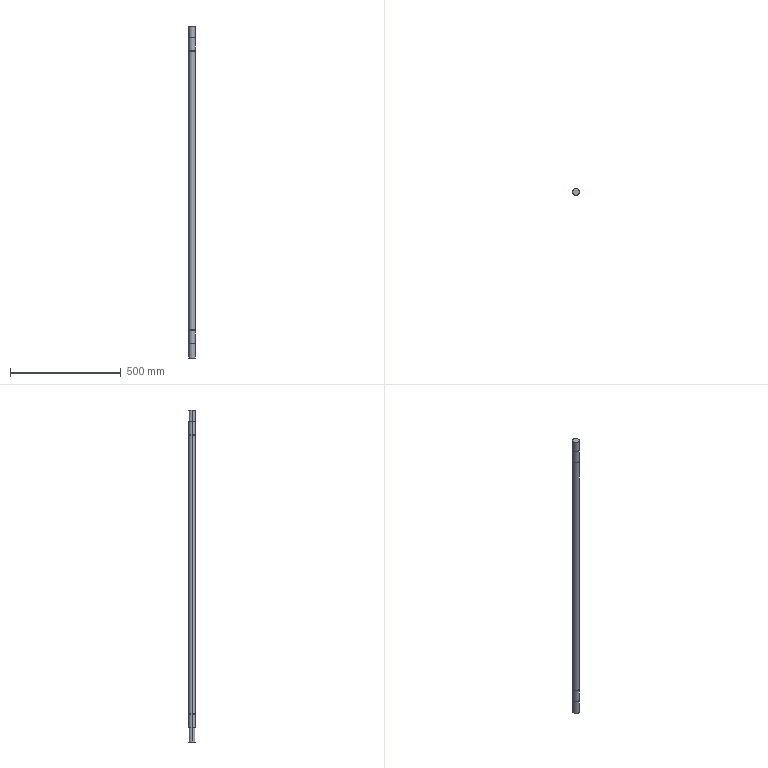Part | SolidWorks | features Extrusion 1, HoleWzd 1, ICE 1, LPattern 1, RevCut 1 | 1 solid | 44 faces | box 30 x 30 x 1500 mm | volume 1054135 mm3 | cylinder 26 | plane 16 | cone 2 | commonest cylinder face diameters 30 x10 28.6 x8 10 x6 6.8 x2
STEP:
#1=CARTESIAN_POINT('',(3.4,0.,19.75));
#2=VERTEX_POINT('',#1);
#3=CARTESIAN_POINT('',(-3.4,0.,19.75));
#4=VERTEX_POINT('',#3);
#5=CARTESIAN_POINT('',(0.,0.,19.75));
#6=DIRECTION('',(0.,0.,-1.));
#7=DIRECTION('',(-1.,0.,0.));
#8=AXIS2_PLACEMENT_3D('',#5,#6,#7);
#9=CIRCLE('',#8,3.4);
#10=EDGE_CURVE('',#2,#4,#9,.T.);
#11=ORIENTED_EDGE('',*,*,#10,.F.);
#12=CARTESIAN_POINT('',(3.4,0.,0.));
#13=VERTEX_POINT('',#12);
#14=CARTESIAN_POINT('',(3.4,0.,0.));
#15=DIRECTION('',(0.,0.,-1.));
#16=VECTOR('',#15,1000.);
#17=LINE('',#14,#16);
#18=EDGE_CURVE('',#2,#13,#17,.T.);
#19=ORIENTED_EDGE('',*,*,#18,.T.);
#20=CARTESIAN_POINT('',(-3.4,0.,0.));
#21=VERTEX_POINT('',#20);
#22=CARTESIAN_POINT('',(0.,0.,0.));
#23=DIRECTION('',(0.,0.,-1.));
#24=DIRECTION('',(-1.,0.,0.));
#25=AXIS2_PLACEMENT_3D('',#22,#23,#24);
#26=CIRCLE('',#25,3.4);
#27=EDGE_CURVE('',#13,#21,#26,.T.);
#28=ORIENTED_EDGE('',*,*,#27,.T.);
#29=CARTESIAN_POINT('',(-3.4,0.,0.));
#30=DIRECTION('',(0.,0.,-1.));
#31=VECTOR('',#30,1000.);
#32=LINE('',#29,#31);
#33=EDGE_CURVE('',#4,#21,#32,.T.);
#34=ORIENTED_EDGE('',*,*,#33,.F.);
#35=EDGE_LOOP('',(#11,#19,#28,#34));
#36=FACE_OUTER_BOUND('',#35,.T.);
#37=CARTESIAN_POINT('',(0.,0.,0.));
#38=DIRECTION('',(0.,0.,-1.));
#39=DIRECTION('',(-1.,0.,0.));
#40=AXIS2_PLACEMENT_3D('',#37,#38,#39);
#41=CYLINDRICAL_SURFACE('',#40,3.4);
#42=ADVANCED_FACE('',(#36),#41,.F.);
#43=CARTESIAN_POINT('',(0.,0.,21.793));
#44=VERTEX_POINT('',#43);
#45=CARTESIAN_POINT('',(-3.4,0.,19.75));
#46=DIRECTION('',(-0.8572,0.,-0.515));
#47=VECTOR('',#46,1000.);
#48=LINE('',#45,#47);
#49=EDGE_CURVE('',#44,#4,#48,.T.);
#50=ORIENTED_EDGE('',*,*,#49,.F.);
#51=CARTESIAN_POINT('',(3.4,0.,19.75));
#52=DIRECTION('',(0.8572,0.,-0.515));
#53=VECTOR('',#52,1000.);
#54=LINE('',#51,#53);
#55=EDGE_CURVE('',#44,#2,#54,.T.);
#56=ORIENTED_EDGE('',*,*,#55,.T.);
#57=ORIENTED_EDGE('',*,*,#10,.T.);
#58=EDGE_LOOP('',(#50,#56,#57));
#59=FACE_OUTER_BOUND('',#58,.T.);
#60=CARTESIAN_POINT('',(0.,0.,19.75));
#61=DIRECTION('',(0.,0.,-1.));
#62=DIRECTION('',(-1.,0.,0.));
#63=AXIS2_PLACEMENT_3D('',#60,#61,#62);
#64=CONICAL_SURFACE('',#63,3.4,1.03);
#65=ADVANCED_FACE('',(#59),#64,.F.);
#66=CARTESIAN_POINT('',(-15.,0.,63.9));
#67=VERTEX_POINT('',#66);
#68=CARTESIAN_POINT('',(15.,0.,63.9));
#69=VERTEX_POINT('',#68);
#70=CARTESIAN_POINT('',(0.,0.,63.9));
#71=DIRECTION('',(0.,0.,-1.));
#72=DIRECTION('',(0.,1.,0.));
#73=AXIS2_PLACEMENT_3D('',#70,#71,#72);
#74=CIRCLE('',#73,15.);
#75=EDGE_CURVE('',#67,#69,#74,.T.);
#76=ORIENTED_EDGE('',*,*,#75,.T.);
#77=CARTESIAN_POINT('',(15.,0.,0.));
#78=VERTEX_POINT('',#77);
#79=CARTESIAN_POINT('',(15.,0.,1500.));
#80=DIRECTION('',(0.,0.,-1.));
#81=VECTOR('',#80,1000.);
#82=LINE('',#79,#81);
#83=EDGE_CURVE('',#69,#78,#82,.T.);
#84=ORIENTED_EDGE('',*,*,#83,.T.);
#85=CARTESIAN_POINT('',(-15.,0.,0.));
#86=VERTEX_POINT('',#85);
#87=CARTESIAN_POINT('',(0.,0.,0.));
#88=DIRECTION('',(0.,0.,1.));
#89=DIRECTION('',(1.,0.,0.));
#90=AXIS2_PLACEMENT_3D('',#87,#88,#89);
#91=CIRCLE('',#90,15.);
#92=EDGE_CURVE('',#78,#86,#91,.T.);
#93=ORIENTED_EDGE('',*,*,#92,.T.);
#94=CARTESIAN_POINT('',(-15.,0.,1500.));
#95=DIRECTION('',(0.,0.,-1.));
#96=VECTOR('',#95,1000.);
#97=LINE('',#94,#96);
#98=EDGE_CURVE('',#67,#86,#97,.T.);
#99=ORIENTED_EDGE('',*,*,#98,.F.);
#100=EDGE_LOOP('',(#76,#84,#93,#99));
#101=FACE_OUTER_BOUND('',#100,.T.);
#102=CARTESIAN_POINT('',(0.,0.,1500.));
#103=DIRECTION('',(0.,0.,-1.));
#104=DIRECTION('',(-1.,0.,0.));
#105=AXIS2_PLACEMENT_3D('',#102,#103,#104);
#106=CYLINDRICAL_SURFACE('',#105,15.);
#107=ADVANCED_FACE('',(#101),#106,.T.);
#108=CARTESIAN_POINT('',(0.,14.3,65.5));
#109=VERTEX_POINT('',#108);
#110=CARTESIAN_POINT('',(0.,-14.3,65.5));
#111=VERTEX_POINT('',#110);
#112=CARTESIAN_POINT('',(0.,0.,65.5));
#113=DIRECTION('',(0.,0.,-1.));
#114=DIRECTION('',(0.,1.,0.));
#115=AXIS2_PLACEMENT_3D('',#112,#113,#114);
#116=CIRCLE('',#115,14.3);
#117=EDGE_CURVE('',#109,#111,#116,.T.);
#118=ORIENTED_EDGE('',*,*,#117,.T.);
#119=CARTESIAN_POINT('',(0.,-14.3,63.9));
#120=VERTEX_POINT('',#119);
#121=CARTESIAN_POINT('',(0.,-14.3,123.));
#122=DIRECTION('',(0.,0.,-1.));
#123=VECTOR('',#122,1000.);
#124=LINE('',#121,#123);
#125=EDGE_CURVE('',#111,#120,#124,.T.);
#126=ORIENTED_EDGE('',*,*,#125,.T.);
#127=CARTESIAN_POINT('',(0.,14.3,63.9));
#128=VERTEX_POINT('',#127);
#129=CARTESIAN_POINT('',(0.,0.,63.9));
#130=DIRECTION('',(0.,0.,-1.));
#131=DIRECTION('',(0.,1.,0.));
#132=AXIS2_PLACEMENT_3D('',#129,#130,#131);
#133=CIRCLE('',#132,14.3);
#134=EDGE_CURVE('',#128,#120,#133,.T.);
#135=ORIENTED_EDGE('',*,*,#134,.F.);
#136=CARTESIAN_POINT('',(0.,14.3,123.));
#137=DIRECTION('',(0.,0.,-1.));
#138=VECTOR('',#137,1000.);
#139=LINE('',#136,#138);
#140=EDGE_CURVE('',#109,#128,#139,.T.);
#141=ORIENTED_EDGE('',*,*,#140,.F.);
#142=EDGE_LOOP('',(#118,#126,#135,#141));
#143=FACE_OUTER_BOUND('',#142,.T.);
#144=CARTESIAN_POINT('',(0.,0.,123.));
#145=DIRECTION('',(0.,0.,-1.));
#146=DIRECTION('',(0.,1.,0.));
#147=AXIS2_PLACEMENT_3D('',#144,#145,#146);
#148=CYLINDRICAL_SURFACE('',#147,14.3);
#149=ADVANCED_FACE('',(#143),#148,.T.);
#150=CARTESIAN_POINT('',(-15.,0.,125.5));
#151=VERTEX_POINT('',#150);
#152=CARTESIAN_POINT('',(15.,0.,125.5));
#153=VERTEX_POINT('',#152);
#154=CARTESIAN_POINT('',(0.,0.,125.5));
#155=DIRECTION('',(0.,0.,-1.));
#156=DIRECTION('',(0.,1.,0.));
#157=AXIS2_PLACEMENT_3D('',#154,#155,#156);
#158=CIRCLE('',#157,15.);
#159=EDGE_CURVE('',#151,#153,#158,.T.);
#160=ORIENTED_EDGE('',*,*,#159,.T.);
#161=CARTESIAN_POINT('',(15.,0.,123.));
#162=VERTEX_POINT('',#161);
#163=CARTESIAN_POINT('',(15.,0.,1500.));
#164=DIRECTION('',(0.,0.,-1.));
#165=VECTOR('',#164,1000.);
#166=LINE('',#163,#165);
#167=EDGE_CURVE('',#153,#162,#166,.T.);
#168=ORIENTED_EDGE('',*,*,#167,.T.);
#169=CARTESIAN_POINT('',(14.142,5.,118.));
#170=VERTEX_POINT('',#169);
#171=CARTESIAN_POINT('',(14.142,5.,118.));
#172=CARTESIAN_POINT('',(14.142,5.,118.33));
#173=CARTESIAN_POINT('',(14.154,4.968,118.656));
#174=CARTESIAN_POINT('',(14.187,4.871,119.14));
#175=CARTESIAN_POINT('',(14.201,4.83,119.302));
#176=CARTESIAN_POINT('',(14.233,4.734,119.617));
#177=CARTESIAN_POINT('',(14.252,4.679,119.771));
#178=CARTESIAN_POINT('',(14.313,4.491,120.222));
#179=CARTESIAN_POINT('',(14.361,4.336,120.511));
#180=CARTESIAN_POINT('',(14.466,3.971,121.055));
#181=CARTESIAN_POINT('',(14.522,3.765,121.305));
#182=CARTESIAN_POINT('',(14.633,3.307,121.764));
#183=CARTESIAN_POINT('',(14.689,3.052,121.974));
#184=CARTESIAN_POINT('',(14.791,2.512,122.336));
#185=CARTESIAN_POINT('',(14.837,2.226,122.489));
#186=CARTESIAN_POINT('',(14.896,1.772,122.678));
#187=CARTESIAN_POINT('',(14.914,1.616,122.735));
#188=CARTESIAN_POINT('',(14.944,1.301,122.831));
#189=CARTESIAN_POINT('',(14.957,1.142,122.871));
#190=CARTESIAN_POINT('',(14.989,0.6599,122.967));
#191=CARTESIAN_POINT('',(15.,0.3329,123.));
#192=CARTESIAN_POINT('',(15.,0.,123.));
#193=B_SPLINE_CURVE_WITH_KNOTS('',3,(#171,#172,#173,#174,#175,#176,#177,#178,#179,#180,#181,#182,#183,#184,#185,#186,#187,#188,#189,#190,#191,#192),.UNSPECIFIED.,.F.,.F.,(4,2,2,2,2,2,2,2,2,2,4),(0.02362,0.0246,0.02509,0.02558,0.02657,0.02755,0.02854,0.02952,0.03001,0.0305,0.03149),.UNSPECIFIED.);
#194=EDGE_CURVE('',#170,#162,#193,.T.);
#195=ORIENTED_EDGE('',*,*,#194,.F.);
#196=CARTESIAN_POINT('',(14.142,5.,73.));
#197=VERTEX_POINT('',#196);
#198=CARTESIAN_POINT('',(14.142,5.,1500.));
#199=DIRECTION('',(0.,0.,1.));
#200=VECTOR('',#199,1000.);
#201=LINE('',#198,#200);
#202=EDGE_CURVE('',#197,#170,#201,.T.);
#203=ORIENTED_EDGE('',*,*,#202,.F.);
#204=CARTESIAN_POINT('',(15.,0.,68.));
#205=VERTEX_POINT('',#204);
#206=CARTESIAN_POINT('',(15.,0.,68.));
#207=CARTESIAN_POINT('',(15.,0.3279,68.));
#208=CARTESIAN_POINT('',(14.989,0.658,68.032));
#209=CARTESIAN_POINT('',(14.947,1.307,68.162));
#210=CARTESIAN_POINT('',(14.915,1.619,68.258));
#211=CARTESIAN_POINT('',(14.838,2.223,68.509));
#212=CARTESIAN_POINT('',(14.79,2.515,68.666));
#213=CARTESIAN_POINT('',(14.688,3.055,69.028));
#214=CARTESIAN_POINT('',(14.633,3.305,69.234));
#215=CARTESIAN_POINT('',(14.521,3.767,69.696));
#216=CARTESIAN_POINT('',(14.465,3.974,69.949));
#217=CARTESIAN_POINT('',(14.361,4.335,70.487));
#218=CARTESIAN_POINT('',(14.313,4.49,70.776));
#219=CARTESIAN_POINT('',(14.231,4.743,71.383));
#220=CARTESIAN_POINT('',(14.199,4.838,71.695));
#221=CARTESIAN_POINT('',(14.154,4.967,72.337));
#222=CARTESIAN_POINT('',(14.142,5.,72.671));
#223=CARTESIAN_POINT('',(14.142,5.,73.));
#224=B_SPLINE_CURVE_WITH_KNOTS('',3,(#206,#207,#208,#209,#210,#211,#212,#213,#214,#215,#216,#217,#218,#219,#220,#221,#222,#223),.UNSPECIFIED.,.F.,.F.,(4,2,2,2,2,2,2,2,4),(0.01575,0.01673,0.01771,0.0187,0.01968,0.02066,0.02165,0.02263,0.02362),.UNSPECIFIED.);
#225=EDGE_CURVE('',#205,#197,#224,.T.);
#226=ORIENTED_EDGE('',*,*,#225,.F.);
#227=CARTESIAN_POINT('',(15.,0.,65.5));
#228=VERTEX_POINT('',#227);
#229=CARTESIAN_POINT('',(15.,0.,1500.));
#230=DIRECTION('',(0.,0.,-1.));
#231=VECTOR('',#230,1000.);
#232=LINE('',#229,#231);
#233=EDGE_CURVE('',#205,#228,#232,.T.);
#234=ORIENTED_EDGE('',*,*,#233,.T.);
#235=CARTESIAN_POINT('',(-15.,0.,65.5));
#236=VERTEX_POINT('',#235);
#237=CARTESIAN_POINT('',(0.,0.,65.5));
#238=DIRECTION('',(0.,0.,-1.));
#239=DIRECTION('',(0.,1.,0.));
#240=AXIS2_PLACEMENT_3D('',#237,#238,#239);
#241=CIRCLE('',#240,15.);
#242=EDGE_CURVE('',#236,#228,#241,.T.);
#243=ORIENTED_EDGE('',*,*,#242,.F.);
#244=CARTESIAN_POINT('',(-15.,0.,1500.));
#245=DIRECTION('',(0.,0.,-1.));
#246=VECTOR('',#245,1000.);
#247=LINE('',#244,#246);
#248=EDGE_CURVE('',#151,#236,#247,.T.);
#249=ORIENTED_EDGE('',*,*,#248,.F.);
#250=EDGE_LOOP('',(#160,#168,#195,#203,#226,#234,#243,#249));
#251=FACE_OUTER_BOUND('',#250,.T.);
#252=CARTESIAN_POINT('',(0.,0.,1500.));
#253=DIRECTION('',(0.,0.,-1.));
#254=DIRECTION('',(-1.,0.,0.));
#255=AXIS2_PLACEMENT_3D('',#252,#253,#254);
#256=CYLINDRICAL_SURFACE('',#255,15.);
#257=ADVANCED_FACE('',(#251),#256,.T.);
#258=ORIENTED_EDGE('',*,*,#194,.T.);
#259=CARTESIAN_POINT('',(10.,0.,123.));
#260=VERTEX_POINT('',#259);
#261=CARTESIAN_POINT('',(15.,0.,123.));
#262=DIRECTION('',(-1.,0.,0.));
#263=VECTOR('',#262,1000.);
#264=LINE('',#261,#263);
#265=EDGE_CURVE('',#162,#260,#264,.T.);
#266=ORIENTED_EDGE('',*,*,#265,.T.);
#267=CARTESIAN_POINT('',(10.,5.,118.));
#268=VERTEX_POINT('',#267);
#269=CARTESIAN_POINT('',(10.,0.,118.));
#270=DIRECTION('',(1.,0.,0.));
#271=DIRECTION('',(0.,0.,-1.));
#272=AXIS2_PLACEMENT_3D('',#269,#270,#271);
#273=CIRCLE('',#272,5.);
#274=EDGE_CURVE('',#268,#260,#273,.T.);
#275=ORIENTED_EDGE('',*,*,#274,.F.);
#276=CARTESIAN_POINT('',(15.,5.,118.));
#277=DIRECTION('',(-1.,0.,0.));
#278=VECTOR('',#277,1000.);
#279=LINE('',#276,#278);
#280=EDGE_CURVE('',#170,#268,#279,.T.);
#281=ORIENTED_EDGE('',*,*,#280,.F.);
#282=EDGE_LOOP('',(#258,#266,#275,#281));
#283=FACE_OUTER_BOUND('',#282,.T.);
#284=CARTESIAN_POINT('',(15.,0.,118.));
#285=DIRECTION('',(-1.,0.,0.));
#286=DIRECTION('',(0.,0.,1.));
#287=AXIS2_PLACEMENT_3D('',#284,#285,#286);
#288=CYLINDRICAL_SURFACE('',#287,5.);
#289=ADVANCED_FACE('',(#283),#288,.F.);
#290=CARTESIAN_POINT('',(0.,14.3,127.1));
#291=VERTEX_POINT('',#290);
#292=CARTESIAN_POINT('',(0.,-14.3,127.1));
#293=VERTEX_POINT('',#292);
#294=CARTESIAN_POINT('',(0.,0.,127.1));
#295=DIRECTION('',(0.,0.,-1.));
#296=DIRECTION('',(0.,1.,0.));
#297=AXIS2_PLACEMENT_3D('',#294,#295,#296);
#298=CIRCLE('',#297,14.3);
#299=EDGE_CURVE('',#291,#293,#298,.T.);
#300=ORIENTED_EDGE('',*,*,#299,.T.);
#301=CARTESIAN_POINT('',(0.,-14.3,125.5));
#302=VERTEX_POINT('',#301);
#303=CARTESIAN_POINT('',(0.,-14.3,123.));
#304=DIRECTION('',(0.,0.,-1.));
#305=VECTOR('',#304,1000.);
#306=LINE('',#303,#305);
#307=EDGE_CURVE('',#293,#302,#306,.T.);
#308=ORIENTED_EDGE('',*,*,#307,.T.);
#309=CARTESIAN_POINT('',(0.,14.3,125.5));
#310=VERTEX_POINT('',#309);
#311=CARTESIAN_POINT('',(0.,0.,125.5));
#312=DIRECTION('',(0.,0.,-1.));
#313=DIRECTION('',(0.,1.,0.));
#314=AXIS2_PLACEMENT_3D('',#311,#312,#313);
#315=CIRCLE('',#314,14.3);
#316=EDGE_CURVE('',#310,#302,#315,.T.);
#317=ORIENTED_EDGE('',*,*,#316,.F.);
#318=CARTESIAN_POINT('',(0.,14.3,123.));
#319=DIRECTION('',(0.,0.,-1.));
#320=VECTOR('',#319,1000.);
#321=LINE('',#318,#320);
#322=EDGE_CURVE('',#291,#310,#321,.T.);
#323=ORIENTED_EDGE('',*,*,#322,.F.);
#324=EDGE_LOOP('',(#300,#308,#317,#323));
#325=FACE_OUTER_BOUND('',#324,.T.);
#326=CARTESIAN_POINT('',(0.,0.,123.));
#327=DIRECTION('',(0.,0.,-1.));
#328=DIRECTION('',(0.,1.,0.));
#329=AXIS2_PLACEMENT_3D('',#326,#327,#328);
#330=CYLINDRICAL_SURFACE('',#329,14.3);
#331=ADVANCED_FACE('',(#325),#330,.T.);
#332=CARTESIAN_POINT('',(15.,0.,1500.));
#333=VERTEX_POINT('',#332);
#334=CARTESIAN_POINT('',(-15.,0.,1500.));
#335=VERTEX_POINT('',#334);
#336=CARTESIAN_POINT('',(0.,0.,1500.));
#337=DIRECTION('',(0.,0.,1.));
#338=DIRECTION('',(1.,0.,0.));
#339=AXIS2_PLACEMENT_3D('',#336,#337,#338);
#340=CIRCLE('',#339,15.);
#341=EDGE_CURVE('',#333,#335,#340,.T.);
#342=ORIENTED_EDGE('',*,*,#341,.F.);
#343=CARTESIAN_POINT('',(15.,0.,1449.1));
#344=VERTEX_POINT('',#343);
#345=CARTESIAN_POINT('',(15.,0.,1500.));
#346=DIRECTION('',(0.,0.,-1.));
#347=VECTOR('',#346,1000.);
#348=LINE('',#345,#347);
#349=EDGE_CURVE('',#333,#344,#348,.T.);
#350=ORIENTED_EDGE('',*,*,#349,.T.);
#351=CARTESIAN_POINT('',(-15.,0.,1449.1));
#352=VERTEX_POINT('',#351);
#353=CARTESIAN_POINT('',(0.,0.,1449.1));
#354=DIRECTION('',(0.,0.,-1.));
#355=DIRECTION('',(0.,1.,0.));
#356=AXIS2_PLACEMENT_3D('',#353,#354,#355);
#357=CIRCLE('',#356,15.);
#358=EDGE_CURVE('',#352,#344,#357,.T.);
#359=ORIENTED_EDGE('',*,*,#358,.F.);
#360=CARTESIAN_POINT('',(-15.,0.,1500.));
#361=DIRECTION('',(0.,0.,-1.));
#362=VECTOR('',#361,1000.);
#363=LINE('',#360,#362);
#364=EDGE_CURVE('',#335,#352,#363,.T.);
#365=ORIENTED_EDGE('',*,*,#364,.F.);
#366=EDGE_LOOP('',(#342,#350,#359,#365));
#367=FACE_OUTER_BOUND('',#366,.T.);
#368=CARTESIAN_POINT('',(0.,0.,1500.));
#369=DIRECTION('',(0.,0.,-1.));
#370=DIRECTION('',(-1.,0.,0.));
#371=AXIS2_PLACEMENT_3D('',#368,#369,#370);
#372=CYLINDRICAL_SURFACE('',#371,15.);
#373=ADVANCED_FACE('',(#367),#372,.T.);
#374=CARTESIAN_POINT('',(0.,14.3,1449.1));
#375=VERTEX_POINT('',#374);
#376=CARTESIAN_POINT('',(0.,-14.3,1449.1));
#377=VERTEX_POINT('',#376);
#378=CARTESIAN_POINT('',(0.,0.,1449.1));
#379=DIRECTION('',(0.,0.,-1.));
#380=DIRECTION('',(0.,1.,0.));
#381=AXIS2_PLACEMENT_3D('',#378,#379,#380);
#382=CIRCLE('',#381,14.3);
#383=EDGE_CURVE('',#375,#377,#382,.T.);
#384=ORIENTED_EDGE('',*,*,#383,.T.);
#385=CARTESIAN_POINT('',(0.,-14.3,1447.5));
#386=VERTEX_POINT('',#385);
#387=CARTESIAN_POINT('',(0.,-14.3,1445.));
#388=DIRECTION('',(0.,0.,-1.));
#389=VECTOR('',#388,1000.);
#390=LINE('',#387,#389);
#391=EDGE_CURVE('',#377,#386,#390,.T.);
#392=ORIENTED_EDGE('',*,*,#391,.T.);
#393=CARTESIAN_POINT('',(0.,14.3,1447.5));
#394=VERTEX_POINT('',#393);
#395=CARTESIAN_POINT('',(0.,0.,1447.5));
#396=DIRECTION('',(0.,0.,-1.));
#397=DIRECTION('',(0.,1.,0.));
#398=AXIS2_PLACEMENT_3D('',#395,#396,#397);
#399=CIRCLE('',#398,14.3);
#400=EDGE_CURVE('',#394,#386,#399,.T.);
#401=ORIENTED_EDGE('',*,*,#400,.F.);
#402=CARTESIAN_POINT('',(0.,14.3,1445.));
#403=DIRECTION('',(0.,0.,-1.));
#404=VECTOR('',#403,1000.);
#405=LINE('',#402,#404);
#406=EDGE_CURVE('',#375,#394,#405,.T.);
#407=ORIENTED_EDGE('',*,*,#406,.F.);
#408=EDGE_LOOP('',(#384,#392,#401,#407));
#409=FACE_OUTER_BOUND('',#408,.T.);
#410=CARTESIAN_POINT('',(0.,0.,1445.));
#411=DIRECTION('',(0.,0.,-1.));
#412=DIRECTION('',(0.,1.,0.));
#413=AXIS2_PLACEMENT_3D('',#410,#411,#412);
#414=CYLINDRICAL_SURFACE('',#413,14.3);
#415=ADVANCED_FACE('',(#409),#414,.T.);
#416=CARTESIAN_POINT('',(0.,14.3,1387.5));
#417=VERTEX_POINT('',#416);
#418=CARTESIAN_POINT('',(0.,-14.3,1387.5));
#419=VERTEX_POINT('',#418);
#420=CARTESIAN_POINT('',(0.,0.,1387.5));
#421=DIRECTION('',(0.,0.,-1.));
#422=DIRECTION('',(0.,1.,0.));
#423=AXIS2_PLACEMENT_3D('',#420,#421,#422);
#424=CIRCLE('',#423,14.3);
#425=EDGE_CURVE('',#417,#419,#424,.T.);
#426=ORIENTED_EDGE('',*,*,#425,.T.);
#427=CARTESIAN_POINT('',(0.,-14.3,1385.9));
#428=VERTEX_POINT('',#427);
#429=CARTESIAN_POINT('',(0.,-14.3,1445.));
#430=DIRECTION('',(0.,0.,-1.));
#431=VECTOR('',#430,1000.);
#432=LINE('',#429,#431);
#433=EDGE_CURVE('',#419,#428,#432,.T.);
#434=ORIENTED_EDGE('',*,*,#433,.T.);
#435=CARTESIAN_POINT('',(0.,14.3,1385.9));
#436=VERTEX_POINT('',#435);
#437=CARTESIAN_POINT('',(0.,0.,1385.9));
#438=DIRECTION('',(0.,0.,-1.));
#439=DIRECTION('',(0.,1.,0.));
#440=AXIS2_PLACEMENT_3D('',#437,#438,#439);
#441=CIRCLE('',#440,14.3);
#442=EDGE_CURVE('',#436,#428,#441,.T.);
#443=ORIENTED_EDGE('',*,*,#442,.F.);
#444=CARTESIAN_POINT('',(0.,14.3,1445.));
#445=DIRECTION('',(0.,0.,-1.));
#446=VECTOR('',#445,1000.);
#447=LINE('',#444,#446);
#448=EDGE_CURVE('',#417,#436,#447,.T.);
#449=ORIENTED_EDGE('',*,*,#448,.F.);
#450=EDGE_LOOP('',(#426,#434,#443,#449));
#451=FACE_OUTER_BOUND('',#450,.T.);
#452=CARTESIAN_POINT('',(0.,0.,1445.));
#453=DIRECTION('',(0.,0.,-1.));
#454=DIRECTION('',(0.,1.,0.));
#455=AXIS2_PLACEMENT_3D('',#452,#453,#454);
#456=CYLINDRICAL_SURFACE('',#455,14.3);
#457=ADVANCED_FACE('',(#451),#456,.T.);
#458=CARTESIAN_POINT('',(14.142,5.,1440.));
#459=VERTEX_POINT('',#458);
#460=CARTESIAN_POINT('',(15.,0.,1445.));
#461=VERTEX_POINT('',#460);
#462=CARTESIAN_POINT('',(14.142,5.,1440.));
#463=CARTESIAN_POINT('',(14.142,5.,1440.33));
#464=CARTESIAN_POINT('',(14.154,4.968,1440.656));
#465=CARTESIAN_POINT('',(14.187,4.871,1441.14));
#466=CARTESIAN_POINT('',(14.201,4.83,1441.302));
#467=CARTESIAN_POINT('',(14.233,4.734,1441.617));
#468=CARTESIAN_POINT('',(14.252,4.679,1441.771));
#469=CARTESIAN_POINT('',(14.313,4.491,1442.222));
#470=CARTESIAN_POINT('',(14.361,4.336,1442.511));
#471=CARTESIAN_POINT('',(14.466,3.971,1443.055));
#472=CARTESIAN_POINT('',(14.522,3.765,1443.305));
#473=CARTESIAN_POINT('',(14.633,3.307,1443.764));
#474=CARTESIAN_POINT('',(14.689,3.052,1443.974));
#475=CARTESIAN_POINT('',(14.791,2.512,1444.336));
#476=CARTESIAN_POINT('',(14.837,2.226,1444.489));
#477=CARTESIAN_POINT('',(14.896,1.772,1444.678));
#478=CARTESIAN_POINT('',(14.914,1.616,1444.735));
#479=CARTESIAN_POINT('',(14.944,1.301,1444.831));
#480=CARTESIAN_POINT('',(14.957,1.142,1444.871));
#481=CARTESIAN_POINT('',(14.989,0.6599,1444.967));
#482=CARTESIAN_POINT('',(15.,0.3329,1445.));
#483=CARTESIAN_POINT('',(15.,0.,1445.));
#484=B_SPLINE_CURVE_WITH_KNOTS('',3,(#462,#463,#464,#465,#466,#467,#468,#469,#470,#471,#472,#473,#474,#475,#476,#477,#478,#479,#480,#481,#482,#483),.UNSPECIFIED.,.F.,.F.,(4,2,2,2,2,2,2,2,2,2,4),(0.02362,0.0246,0.02509,0.02558,0.02657,0.02755,0.02854,0.02952,0.03001,0.0305,0.03149),.UNSPECIFIED.);
#485=EDGE_CURVE('',#459,#461,#484,.T.);
#486=ORIENTED_EDGE('',*,*,#485,.T.);
#487=CARTESIAN_POINT('',(10.,0.,1445.));
#488=VERTEX_POINT('',#487);
#489=CARTESIAN_POINT('',(15.,0.,1445.));
#490=DIRECTION('',(-1.,0.,0.));
#491=VECTOR('',#490,1000.);
#492=LINE('',#489,#491);
#493=EDGE_CURVE('',#461,#488,#492,.T.);
#494=ORIENTED_EDGE('',*,*,#493,.T.);
#495=CARTESIAN_POINT('',(10.,5.,1440.));
#496=VERTEX_POINT('',#495);
#497=CARTESIAN_POINT('',(10.,0.,1440.));
#498=DIRECTION('',(1.,0.,0.));
#499=DIRECTION('',(0.,0.,-1.));
#500=AXIS2_PLACEMENT_3D('',#497,#498,#499);
#501=CIRCLE('',#500,5.);
#502=EDGE_CURVE('',#496,#488,#501,.T.);
#503=ORIENTED_EDGE('',*,*,#502,.F.);
#504=CARTESIAN_POINT('',(15.,5.,1440.));
#505=DIRECTION('',(-1.,0.,0.));
#506=VECTOR('',#505,1000.);
#507=LINE('',#504,#506);
#508=EDGE_CURVE('',#459,#496,#507,.T.);
#509=ORIENTED_EDGE('',*,*,#508,.F.);
#510=EDGE_LOOP('',(#486,#494,#503,#509));
#511=FACE_OUTER_BOUND('',#510,.T.);
#512=CARTESIAN_POINT('',(15.,0.,1440.));
#513=DIRECTION('',(-1.,0.,0.));
#514=DIRECTION('',(0.,0.,1.));
#515=AXIS2_PLACEMENT_3D('',#512,#513,#514);
#516=CYLINDRICAL_SURFACE('',#515,5.);
#517=ADVANCED_FACE('',(#511),#516,.F.);
#518=CARTESIAN_POINT('',(-15.,0.,1447.5));
#519=VERTEX_POINT('',#518);
#520=CARTESIAN_POINT('',(15.,0.,1447.5));
#521=VERTEX_POINT('',#520);
#522=CARTESIAN_POINT('',(0.,0.,1447.5));
#523=DIRECTION('',(0.,0.,-1.));
#524=DIRECTION('',(0.,1.,0.));
#525=AXIS2_PLACEMENT_3D('',#522,#523,#524);
#526=CIRCLE('',#525,15.);
#527=EDGE_CURVE('',#519,#521,#526,.T.);
#528=ORIENTED_EDGE('',*,*,#527,.T.);
#529=CARTESIAN_POINT('',(15.,0.,1500.));
#530=DIRECTION('',(0.,0.,-1.));
#531=VECTOR('',#530,1000.);
#532=LINE('',#529,#531);
#533=EDGE_CURVE('',#521,#461,#532,.T.);
#534=ORIENTED_EDGE('',*,*,#533,.T.);
#535=ORIENTED_EDGE('',*,*,#485,.F.);
#536=CARTESIAN_POINT('',(14.142,5.,1395.));
#537=VERTEX_POINT('',#536);
#538=CARTESIAN_POINT('',(14.142,5.,1500.));
#539=DIRECTION('',(0.,0.,1.));
#540=VECTOR('',#539,1000.);
#541=LINE('',#538,#540);
#542=EDGE_CURVE('',#537,#459,#541,.T.);
#543=ORIENTED_EDGE('',*,*,#542,.F.);
#544=CARTESIAN_POINT('',(15.,0.,1390.));
#545=VERTEX_POINT('',#544);
#546=CARTESIAN_POINT('',(15.,0.,1390.));
#547=CARTESIAN_POINT('',(15.,0.3279,1390.));
#548=CARTESIAN_POINT('',(14.989,0.658,1390.032));
#549=CARTESIAN_POINT('',(14.947,1.307,1390.162));
#550=CARTESIAN_POINT('',(14.915,1.619,1390.258));
#551=CARTESIAN_POINT('',(14.838,2.223,1390.509));
#552=CARTESIAN_POINT('',(14.79,2.515,1390.666));
#553=CARTESIAN_POINT('',(14.688,3.055,1391.028));
#554=CARTESIAN_POINT('',(14.633,3.305,1391.234));
#555=CARTESIAN_POINT('',(14.521,3.767,1391.696));
#556=CARTESIAN_POINT('',(14.465,3.974,1391.949));
#557=CARTESIAN_POINT('',(14.361,4.335,1392.487));
#558=CARTESIAN_POINT('',(14.313,4.49,1392.776));
#559=CARTESIAN_POINT('',(14.231,4.743,1393.383));
#560=CARTESIAN_POINT('',(14.199,4.838,1393.695));
#561=CARTESIAN_POINT('',(14.154,4.967,1394.337));
#562=CARTESIAN_POINT('',(14.142,5.,1394.671));
#563=CARTESIAN_POINT('',(14.142,5.,1395.));
#564=B_SPLINE_CURVE_WITH_KNOTS('',3,(#546,#547,#548,#549,#550,#551,#552,#553,#554,#555,#556,#557,#558,#559,#560,#561,#562,#563),.UNSPECIFIED.,.F.,.F.,(4,2,2,2,2,2,2,2,4),(0.01575,0.01673,0.01771,0.0187,0.01968,0.02066,0.02165,0.02263,0.02362),.UNSPECIFIED.);
#565=EDGE_CURVE('',#545,#537,#564,.T.);
#566=ORIENTED_EDGE('',*,*,#565,.F.);
#567=CARTESIAN_POINT('',(15.,0.,1387.5));
#568=VERTEX_POINT('',#567);
#569=CARTESIAN_POINT('',(15.,0.,1500.));
#570=DIRECTION('',(0.,0.,-1.));
#571=VECTOR('',#570,1000.);
#572=LINE('',#569,#571);
#573=EDGE_CURVE('',#545,#568,#572,.T.);
#574=ORIENTED_EDGE('',*,*,#573,.T.);
#575=CARTESIAN_POINT('',(-15.,0.,1387.5));
#576=VERTEX_POINT('',#575);
#577=CARTESIAN_POINT('',(0.,0.,1387.5));
#578=DIRECTION('',(0.,0.,-1.));
#579=DIRECTION('',(0.,1.,0.));
#580=AXIS2_PLACEMENT_3D('',#577,#578,#579);
#581=CIRCLE('',#580,15.);
#582=EDGE_CURVE('',#576,#568,#581,.T.);
#583=ORIENTED_EDGE('',*,*,#582,.F.);
#584=CARTESIAN_POINT('',(-15.,0.,1500.));
#585=DIRECTION('',(0.,0.,-1.));
#586=VECTOR('',#585,1000.);
#587=LINE('',#584,#586);
#588=EDGE_CURVE('',#519,#576,#587,.T.);
#589=ORIENTED_EDGE('',*,*,#588,.F.);
#590=EDGE_LOOP('',(#528,#534,#535,#543,#566,#574,#583,#589));
#591=FACE_OUTER_BOUND('',#590,.T.);
#592=CARTESIAN_POINT('',(0.,0.,1500.));
#593=DIRECTION('',(0.,0.,-1.));
#594=DIRECTION('',(-1.,0.,0.));
#595=AXIS2_PLACEMENT_3D('',#592,#593,#594);
#596=CYLINDRICAL_SURFACE('',#595,15.);
#597=ADVANCED_FACE('',(#591),#596,.T.);
#598=CARTESIAN_POINT('',(-15.,0.,1385.9));
#599=VERTEX_POINT('',#598);
#600=CARTESIAN_POINT('',(15.,0.,1385.9));
#601=VERTEX_POINT('',#600);
#602=CARTESIAN_POINT('',(0.,0.,1385.9));
#603=DIRECTION('',(0.,0.,-1.));
#604=DIRECTION('',(0.,1.,0.));
#605=AXIS2_PLACEMENT_3D('',#602,#603,#604);
#606=CIRCLE('',#605,15.);
#607=EDGE_CURVE('',#599,#601,#606,.T.);
#608=ORIENTED_EDGE('',*,*,#607,.T.);
#609=CARTESIAN_POINT('',(15.,0.,127.1));
#610=VERTEX_POINT('',#609);
#611=CARTESIAN_POINT('',(15.,0.,1500.));
#612=DIRECTION('',(0.,0.,-1.));
#613=VECTOR('',#612,1000.);
#614=LINE('',#611,#613);
#615=EDGE_CURVE('',#601,#610,#614,.T.);
#616=ORIENTED_EDGE('',*,*,#615,.T.);
#617=CARTESIAN_POINT('',(-15.,0.,127.1));
#618=VERTEX_POINT('',#617);
#619=CARTESIAN_POINT('',(0.,0.,127.1));
#620=DIRECTION('',(0.,0.,-1.));
#621=DIRECTION('',(0.,1.,0.));
#622=AXIS2_PLACEMENT_3D('',#619,#620,#621);
#623=CIRCLE('',#622,15.);
#624=EDGE_CURVE('',#618,#610,#623,.T.);
#625=ORIENTED_EDGE('',*,*,#624,.F.);
#626=CARTESIAN_POINT('',(-15.,0.,1500.));
#627=DIRECTION('',(0.,0.,-1.));
#628=VECTOR('',#627,1000.);
#629=LINE('',#626,#628);
#630=EDGE_CURVE('',#599,#618,#629,.T.);
#631=ORIENTED_EDGE('',*,*,#630,.F.);
#632=EDGE_LOOP('',(#608,#616,#625,#631));
#633=FACE_OUTER_BOUND('',#632,.T.);
#634=CARTESIAN_POINT('',(0.,0.,1500.));
#635=DIRECTION('',(0.,0.,-1.));
#636=DIRECTION('',(-1.,0.,0.));
#637=AXIS2_PLACEMENT_3D('',#634,#635,#636);
#638=CYLINDRICAL_SURFACE('',#637,15.);
#639=ADVANCED_FACE('',(#633),#638,.T.);
#640=ORIENTED_EDGE('',*,*,#615,.F.);
#641=CARTESIAN_POINT('',(0.,0.,1385.9));
#642=DIRECTION('',(0.,0.,-1.));
#643=DIRECTION('',(0.,1.,0.));
#644=AXIS2_PLACEMENT_3D('',#641,#642,#643);
#645=CIRCLE('',#644,15.);
#646=EDGE_CURVE('',#601,#599,#645,.T.);
#647=ORIENTED_EDGE('',*,*,#646,.T.);
#648=ORIENTED_EDGE('',*,*,#630,.T.);
#649=CARTESIAN_POINT('',(0.,0.,127.1));
#650=DIRECTION('',(0.,0.,-1.));
#651=DIRECTION('',(0.,1.,0.));
#652=AXIS2_PLACEMENT_3D('',#649,#650,#651);
#653=CIRCLE('',#652,15.);
#654=EDGE_CURVE('',#610,#618,#653,.T.);
#655=ORIENTED_EDGE('',*,*,#654,.F.);
#656=EDGE_LOOP('',(#640,#647,#648,#655));
#657=FACE_OUTER_BOUND('',#656,.T.);
#658=CARTESIAN_POINT('',(0.,0.,1500.));
#659=DIRECTION('',(0.,0.,-1.));
#660=DIRECTION('',(-1.,0.,0.));
#661=AXIS2_PLACEMENT_3D('',#658,#659,#660);
#662=CYLINDRICAL_SURFACE('',#661,15.);
#663=ADVANCED_FACE('',(#657),#662,.T.);
#664=ORIENTED_EDGE('',*,*,#533,.F.);
#665=CARTESIAN_POINT('',(0.,0.,1447.5));
#666=DIRECTION('',(0.,0.,-1.));
#667=DIRECTION('',(0.,1.,0.));
#668=AXIS2_PLACEMENT_3D('',#665,#666,#667);
#669=CIRCLE('',#668,15.);
#670=EDGE_CURVE('',#521,#519,#669,.T.);
#671=ORIENTED_EDGE('',*,*,#670,.T.);
#672=ORIENTED_EDGE('',*,*,#588,.T.);
#673=CARTESIAN_POINT('',(0.,0.,1387.5));
#674=DIRECTION('',(0.,0.,-1.));
#675=DIRECTION('',(0.,1.,0.));
#676=AXIS2_PLACEMENT_3D('',#673,#674,#675);
#677=CIRCLE('',#676,15.);
#678=EDGE_CURVE('',#568,#576,#677,.T.);
#679=ORIENTED_EDGE('',*,*,#678,.F.);
#680=ORIENTED_EDGE('',*,*,#573,.F.);
#681=CARTESIAN_POINT('',(14.142,-5.,1395.));
#682=VERTEX_POINT('',#681);
#683=CARTESIAN_POINT('',(14.142,-5.,1395.));
#684=CARTESIAN_POINT('',(14.142,-5.,1394.671));
#685=CARTESIAN_POINT('',(14.154,-4.967,1394.337));
#686=CARTESIAN_POINT('',(14.199,-4.838,1393.694));
#687=CARTESIAN_POINT('',(14.231,-4.742,1393.382));
#688=CARTESIAN_POINT('',(14.313,-4.489,1392.773));
#689=CARTESIAN_POINT('',(14.362,-4.334,1392.485));
#690=CARTESIAN_POINT('',(14.466,-3.973,1391.947));
#691=CARTESIAN_POINT('',(14.522,-3.764,1391.692));
#692=CARTESIAN_POINT('',(14.634,-3.303,1391.232));
#693=CARTESIAN_POINT('',(14.689,-3.053,1391.027));
#694=CARTESIAN_POINT('',(14.791,-2.513,1390.665));
#695=CARTESIAN_POINT('',(14.838,-2.22,1390.508));
#696=CARTESIAN_POINT('',(14.916,-1.618,1390.258));
#697=CARTESIAN_POINT('',(14.947,-1.306,1390.162));
#698=CARTESIAN_POINT('',(14.978,-0.821,1390.065));
#699=CARTESIAN_POINT('',(14.987,-0.656,1390.04));
#700=CARTESIAN_POINT('',(14.997,-0.3279,1390.008));
#701=CARTESIAN_POINT('',(15.,-0.1639,1390.));
#702=CARTESIAN_POINT('',(15.,0.,1390.));
#703=B_SPLINE_CURVE_WITH_KNOTS('',3,(#683,#684,#685,#686,#687,#688,#689,#690,#691,#692,#693,#694,#695,#696,#697,#698,#699,#700,#701,#702),.UNSPECIFIED.,.F.,.F.,(4,2,2,2,2,2,2,2,2,4),(0.007875,0.008859,0.009843,0.01083,0.01181,0.01279,0.01378,0.01476,0.01525,0.01575),.UNSPECIFIED.);
#704=EDGE_CURVE('',#682,#545,#703,.T.);
#705=ORIENTED_EDGE('',*,*,#704,.F.);
#706=CARTESIAN_POINT('',(14.142,-5.,1440.));
#707=VERTEX_POINT('',#706);
#708=CARTESIAN_POINT('',(14.142,-5.,1500.));
#709=DIRECTION('',(0.,0.,-1.));
#710=VECTOR('',#709,1000.);
#711=LINE('',#708,#710);
#712=EDGE_CURVE('',#707,#682,#711,.T.);
#713=ORIENTED_EDGE('',*,*,#712,.F.);
#714=CARTESIAN_POINT('',(15.,0.,1445.));
#715=CARTESIAN_POINT('',(15.,-0.333,1445.));
#716=CARTESIAN_POINT('',(14.989,-0.66,1444.967));
#717=CARTESIAN_POINT('',(14.947,-1.303,1444.838));
#718=CARTESIAN_POINT('',(14.915,-1.622,1444.741));
#719=CARTESIAN_POINT('',(14.837,-2.226,1444.489));
#720=CARTESIAN_POINT('',(14.791,-2.513,1444.335));
#721=CARTESIAN_POINT('',(14.688,-3.055,1443.972));
#722=CARTESIAN_POINT('',(14.632,-3.309,1443.762));
#723=CARTESIAN_POINT('',(14.521,-3.767,1443.304));
#724=CARTESIAN_POINT('',(14.466,-3.973,1443.054));
#725=CARTESIAN_POINT('',(14.36,-4.338,1442.508));
#726=CARTESIAN_POINT('',(14.312,-4.492,1442.221));
#727=CARTESIAN_POINT('',(14.252,-4.679,1441.77));
#728=CARTESIAN_POINT('',(14.233,-4.734,1441.616));
#729=CARTESIAN_POINT('',(14.201,-4.83,1441.302));
#730=CARTESIAN_POINT('',(14.187,-4.871,1441.14));
#731=CARTESIAN_POINT('',(14.154,-4.968,1440.655));
#732=CARTESIAN_POINT('',(14.142,-5.,1440.329));
#733=CARTESIAN_POINT('',(14.142,-5.,1440.));
#734=B_SPLINE_CURVE_WITH_KNOTS('',3,(#714,#715,#716,#717,#718,#719,#720,#721,#722,#723,#724,#725,#726,#727,#728,#729,#730,#731,#732,#733),.UNSPECIFIED.,.F.,.F.,(4,2,2,2,2,2,2,2,2,4),(0.,0.0009844,0.001969,0.002953,0.003938,0.004922,0.005907,0.006399,0.006891,0.007875),.UNSPECIFIED.);
#735=EDGE_CURVE('',#461,#707,#734,.T.);
#736=ORIENTED_EDGE('',*,*,#735,.F.);
#737=EDGE_LOOP('',(#664,#671,#672,#679,#680,#705,#713,#736));
#738=FACE_OUTER_BOUND('',#737,.T.);
#739=CARTESIAN_POINT('',(0.,0.,1500.));
#740=DIRECTION('',(0.,0.,-1.));
#741=DIRECTION('',(-1.,0.,0.));
#742=AXIS2_PLACEMENT_3D('',#739,#740,#741);
#743=CYLINDRICAL_SURFACE('',#742,15.);
#744=ADVANCED_FACE('',(#738),#743,.T.);
#745=ORIENTED_EDGE('',*,*,#493,.F.);
#746=ORIENTED_EDGE('',*,*,#735,.T.);
#747=CARTESIAN_POINT('',(10.,-5.,1440.));
#748=VERTEX_POINT('',#747);
#749=CARTESIAN_POINT('',(15.,-5.,1440.));
#750=DIRECTION('',(-1.,0.,0.));
#751=VECTOR('',#750,1000.);
#752=LINE('',#749,#751);
#753=EDGE_CURVE('',#707,#748,#752,.T.);
#754=ORIENTED_EDGE('',*,*,#753,.T.);
#755=CARTESIAN_POINT('',(10.,0.,1440.));
#756=DIRECTION('',(1.,0.,0.));
#757=DIRECTION('',(0.,0.,-1.));
#758=AXIS2_PLACEMENT_3D('',#755,#756,#757);
#759=CIRCLE('',#758,5.);
#760=EDGE_CURVE('',#488,#748,#759,.T.);
#761=ORIENTED_EDGE('',*,*,#760,.F.);
#762=EDGE_LOOP('',(#745,#746,#754,#761));
#763=FACE_OUTER_BOUND('',#762,.T.);
#764=CARTESIAN_POINT('',(15.,0.,1440.));
#765=DIRECTION('',(-1.,0.,0.));
#766=DIRECTION('',(0.,0.,1.));
#767=AXIS2_PLACEMENT_3D('',#764,#765,#766);
#768=CYLINDRICAL_SURFACE('',#767,5.);
#769=ADVANCED_FACE('',(#763),#768,.F.);
#770=ORIENTED_EDGE('',*,*,#712,.T.);
#771=CARTESIAN_POINT('',(10.,-5.,1395.));
#772=VERTEX_POINT('',#771);
#773=CARTESIAN_POINT('',(15.,-5.,1395.));
#774=DIRECTION('',(-1.,0.,0.));
#775=VECTOR('',#774,1000.);
#776=LINE('',#773,#775);
#777=EDGE_CURVE('',#682,#772,#776,.T.);
#778=ORIENTED_EDGE('',*,*,#777,.T.);
#779=CARTESIAN_POINT('',(10.,-5.,1440.));
#780=DIRECTION('',(0.,0.,-1.));
#781=VECTOR('',#780,1000.);
#782=LINE('',#779,#781);
#783=EDGE_CURVE('',#748,#772,#782,.T.);
#784=ORIENTED_EDGE('',*,*,#783,.F.);
#785=ORIENTED_EDGE('',*,*,#753,.F.);
#786=EDGE_LOOP('',(#770,#778,#784,#785));
#787=FACE_OUTER_BOUND('',#786,.T.);
#788=CARTESIAN_POINT('',(15.,-5.,1440.));
#789=DIRECTION('',(0.,1.,0.));
#790=DIRECTION('',(0.,0.,1.));
#791=AXIS2_PLACEMENT_3D('',#788,#789,#790);
#792=PLANE('',#791);
#793=ADVANCED_FACE('',(#787),#792,.T.);
#794=ORIENTED_EDGE('',*,*,#777,.F.);
#795=ORIENTED_EDGE('',*,*,#704,.T.);
#796=ORIENTED_EDGE('',*,*,#565,.T.);
#797=CARTESIAN_POINT('',(10.,5.,1395.));
#798=VERTEX_POINT('',#797);
#799=CARTESIAN_POINT('',(15.,5.,1395.));
#800=DIRECTION('',(-1.,0.,0.));
#801=VECTOR('',#800,1000.);
#802=LINE('',#799,#801);
#803=EDGE_CURVE('',#537,#798,#802,.T.);
#804=ORIENTED_EDGE('',*,*,#803,.T.);
#805=CARTESIAN_POINT('',(10.,0.,1395.));
#806=DIRECTION('',(1.,0.,0.));
#807=DIRECTION('',(0.,0.,-1.));
#808=AXIS2_PLACEMENT_3D('',#805,#806,#807);
#809=CIRCLE('',#808,5.);
#810=EDGE_CURVE('',#772,#798,#809,.T.);
#811=ORIENTED_EDGE('',*,*,#810,.F.);
#812=EDGE_LOOP('',(#794,#795,#796,#804,#811));
#813=FACE_OUTER_BOUND('',#812,.T.);
#814=CARTESIAN_POINT('',(15.,0.,1395.));
#815=DIRECTION('',(-1.,0.,0.));
#816=DIRECTION('',(0.,0.,1.));
#817=AXIS2_PLACEMENT_3D('',#814,#815,#816);
#818=CYLINDRICAL_SURFACE('',#817,5.);
#819=ADVANCED_FACE('',(#813),#818,.F.);
#820=ORIENTED_EDGE('',*,*,#542,.T.);
#821=ORIENTED_EDGE('',*,*,#508,.T.);
#822=CARTESIAN_POINT('',(10.,5.,1440.));
#823=DIRECTION('',(0.,0.,1.));
#824=VECTOR('',#823,1000.);
#825=LINE('',#822,#824);
#826=EDGE_CURVE('',#798,#496,#825,.T.);
#827=ORIENTED_EDGE('',*,*,#826,.F.);
#828=ORIENTED_EDGE('',*,*,#803,.F.);
#829=EDGE_LOOP('',(#820,#821,#827,#828));
#830=FACE_OUTER_BOUND('',#829,.T.);
#831=CARTESIAN_POINT('',(15.,5.,1440.));
#832=DIRECTION('',(0.,-1.,0.));
#833=DIRECTION('',(0.,0.,-1.));
#834=AXIS2_PLACEMENT_3D('',#831,#832,#833);
#835=PLANE('',#834);
#836=ADVANCED_FACE('',(#830),#835,.T.);
#837=ORIENTED_EDGE('',*,*,#502,.T.);
#838=ORIENTED_EDGE('',*,*,#760,.T.);
#839=ORIENTED_EDGE('',*,*,#783,.T.);
#840=ORIENTED_EDGE('',*,*,#810,.T.);
#841=ORIENTED_EDGE('',*,*,#826,.T.);
#842=EDGE_LOOP('',(#837,#838,#839,#840,#841));
#843=FACE_OUTER_BOUND('',#842,.T.);
#844=CARTESIAN_POINT('',(10.,0.,1440.));
#845=DIRECTION('',(1.,0.,0.));
#846=DIRECTION('',(0.,0.,-1.));
#847=AXIS2_PLACEMENT_3D('',#844,#845,#846);
#848=PLANE('',#847);
#849=ADVANCED_FACE('',(#843),#848,.T.);
#850=ORIENTED_EDGE('',*,*,#425,.F.);
#851=CARTESIAN_POINT('',(0.,0.,1387.5));
#852=DIRECTION('',(0.,0.,-1.));
#853=DIRECTION('',(0.,1.,0.));
#854=AXIS2_PLACEMENT_3D('',#851,#852,#853);
#855=CIRCLE('',#854,14.3);
#856=EDGE_CURVE('',#419,#417,#855,.T.);
#857=ORIENTED_EDGE('',*,*,#856,.F.);
#858=EDGE_LOOP('',(#850,#857));
#859=FACE_BOUND('',#858,.T.);
#860=ORIENTED_EDGE('',*,*,#582,.T.);
#861=ORIENTED_EDGE('',*,*,#678,.T.);
#862=EDGE_LOOP('',(#860,#861));
#863=FACE_OUTER_BOUND('',#862,.T.);
#864=CARTESIAN_POINT('',(0.,15.,1387.5));
#865=DIRECTION('',(0.,0.,1.));
#866=DIRECTION('',(0.,-1.,0.));
#867=AXIS2_PLACEMENT_3D('',#864,#865,#866);
#868=PLANE('',#867);
#869=ADVANCED_FACE('',(#859,#863),#868,.F.);
#870=ORIENTED_EDGE('',*,*,#433,.F.);
#871=ORIENTED_EDGE('',*,*,#856,.T.);
#872=ORIENTED_EDGE('',*,*,#448,.T.);
#873=CARTESIAN_POINT('',(0.,0.,1385.9));
#874=DIRECTION('',(0.,0.,-1.));
#875=DIRECTION('',(0.,1.,0.));
#876=AXIS2_PLACEMENT_3D('',#873,#874,#875);
#877=CIRCLE('',#876,14.3);
#878=EDGE_CURVE('',#428,#436,#877,.T.);
#879=ORIENTED_EDGE('',*,*,#878,.F.);
#880=EDGE_LOOP('',(#870,#871,#872,#879));
#881=FACE_OUTER_BOUND('',#880,.T.);
#882=CARTESIAN_POINT('',(0.,0.,1445.));
#883=DIRECTION('',(0.,0.,-1.));
#884=DIRECTION('',(0.,1.,0.));
#885=AXIS2_PLACEMENT_3D('',#882,#883,#884);
#886=CYLINDRICAL_SURFACE('',#885,14.3);
#887=ADVANCED_FACE('',(#881),#886,.T.);
#888=ORIENTED_EDGE('',*,*,#607,.F.);
#889=ORIENTED_EDGE('',*,*,#646,.F.);
#890=EDGE_LOOP('',(#888,#889));
#891=FACE_OUTER_BOUND('',#890,.T.);
#892=ORIENTED_EDGE('',*,*,#442,.T.);
#893=ORIENTED_EDGE('',*,*,#878,.T.);
#894=EDGE_LOOP('',(#892,#893));
#895=FACE_BOUND('',#894,.T.);
#896=CARTESIAN_POINT('',(0.,15.,1385.9));
#897=DIRECTION('',(0.,0.,-1.));
#898=DIRECTION('',(0.,1.,0.));
#899=AXIS2_PLACEMENT_3D('',#896,#897,#898);
#900=PLANE('',#899);
#901=ADVANCED_FACE('',(#891,#895),#900,.F.);
#902=ORIENTED_EDGE('',*,*,#383,.F.);
#903=CARTESIAN_POINT('',(0.,0.,1449.1));
#904=DIRECTION('',(0.,0.,-1.));
#905=DIRECTION('',(0.,1.,0.));
#906=AXIS2_PLACEMENT_3D('',#903,#904,#905);
#907=CIRCLE('',#906,14.3);
#908=EDGE_CURVE('',#377,#375,#907,.T.);
#909=ORIENTED_EDGE('',*,*,#908,.F.);
#910=EDGE_LOOP('',(#902,#909));
#911=FACE_BOUND('',#910,.T.);
#912=ORIENTED_EDGE('',*,*,#358,.T.);
#913=CARTESIAN_POINT('',(0.,0.,1449.1));
#914=DIRECTION('',(0.,0.,-1.));
#915=DIRECTION('',(0.,1.,0.));
#916=AXIS2_PLACEMENT_3D('',#913,#914,#915);
#917=CIRCLE('',#916,15.);
#918=EDGE_CURVE('',#344,#352,#917,.T.);
#919=ORIENTED_EDGE('',*,*,#918,.T.);
#920=EDGE_LOOP('',(#912,#919));
#921=FACE_OUTER_BOUND('',#920,.T.);
#922=CARTESIAN_POINT('',(0.,15.,1449.1));
#923=DIRECTION('',(0.,0.,1.));
#924=DIRECTION('',(0.,-1.,0.));
#925=AXIS2_PLACEMENT_3D('',#922,#923,#924);
#926=PLANE('',#925);
#927=ADVANCED_FACE('',(#911,#921),#926,.F.);
#928=ORIENTED_EDGE('',*,*,#391,.F.);
#929=ORIENTED_EDGE('',*,*,#908,.T.);
#930=ORIENTED_EDGE('',*,*,#406,.T.);
#931=CARTESIAN_POINT('',(0.,0.,1447.5));
#932=DIRECTION('',(0.,0.,-1.));
#933=DIRECTION('',(0.,1.,0.));
#934=AXIS2_PLACEMENT_3D('',#931,#932,#933);
#935=CIRCLE('',#934,14.3);
#936=EDGE_CURVE('',#386,#394,#935,.T.);
#937=ORIENTED_EDGE('',*,*,#936,.F.);
#938=EDGE_LOOP('',(#928,#929,#930,#937));
#939=FACE_OUTER_BOUND('',#938,.T.);
#940=CARTESIAN_POINT('',(0.,0.,1445.));
#941=DIRECTION('',(0.,0.,-1.));
#942=DIRECTION('',(0.,1.,0.));
#943=AXIS2_PLACEMENT_3D('',#940,#941,#942);
#944=CYLINDRICAL_SURFACE('',#943,14.3);
#945=ADVANCED_FACE('',(#939),#944,.T.);
#946=ORIENTED_EDGE('',*,*,#527,.F.);
#947=ORIENTED_EDGE('',*,*,#670,.F.);
#948=EDGE_LOOP('',(#946,#947));
#949=FACE_OUTER_BOUND('',#948,.T.);
#950=ORIENTED_EDGE('',*,*,#400,.T.);
#951=ORIENTED_EDGE('',*,*,#936,.T.);
#952=EDGE_LOOP('',(#950,#951));
#953=FACE_BOUND('',#952,.T.);
#954=CARTESIAN_POINT('',(0.,15.,1447.5));
#955=DIRECTION('',(0.,0.,-1.));
#956=DIRECTION('',(0.,1.,0.));
#957=AXIS2_PLACEMENT_3D('',#954,#955,#956);
#958=PLANE('',#957);
#959=ADVANCED_FACE('',(#949,#953),#958,.F.);
#960=CARTESIAN_POINT('',(0.,0.,1500.));
#961=DIRECTION('',(0.,0.,1.));
#962=DIRECTION('',(1.,0.,0.));
#963=AXIS2_PLACEMENT_3D('',#960,#961,#962);
#964=CIRCLE('',#963,15.);
#965=EDGE_CURVE('',#335,#333,#964,.T.);
#966=ORIENTED_EDGE('',*,*,#965,.T.);
#967=ORIENTED_EDGE('',*,*,#341,.T.);
#968=EDGE_LOOP('',(#966,#967));
#969=FACE_OUTER_BOUND('',#968,.T.);
#970=CARTESIAN_POINT('',(0.,0.,1500.));
#971=DIRECTION('',(0.,0.,1.));
#972=DIRECTION('',(1.,0.,0.));
#973=AXIS2_PLACEMENT_3D('',#970,#971,#972);
#974=PLANE('',#973);
#975=ADVANCED_FACE('',(#969),#974,.T.);
#976=ORIENTED_EDGE('',*,*,#349,.F.);
#977=ORIENTED_EDGE('',*,*,#965,.F.);
#978=ORIENTED_EDGE('',*,*,#364,.T.);
#979=ORIENTED_EDGE('',*,*,#918,.F.);
#980=EDGE_LOOP('',(#976,#977,#978,#979));
#981=FACE_OUTER_BOUND('',#980,.T.);
#982=CARTESIAN_POINT('',(0.,0.,1500.));
#983=DIRECTION('',(0.,0.,-1.));
#984=DIRECTION('',(-1.,0.,0.));
#985=AXIS2_PLACEMENT_3D('',#982,#983,#984);
#986=CYLINDRICAL_SURFACE('',#985,15.);
#987=ADVANCED_FACE('',(#981),#986,.T.);
#988=ORIENTED_EDGE('',*,*,#299,.F.);
#989=CARTESIAN_POINT('',(0.,0.,127.1));
#990=DIRECTION('',(0.,0.,-1.));
#991=DIRECTION('',(0.,1.,0.));
#992=AXIS2_PLACEMENT_3D('',#989,#990,#991);
#993=CIRCLE('',#992,14.3);
#994=EDGE_CURVE('',#293,#291,#993,.T.);
#995=ORIENTED_EDGE('',*,*,#994,.F.);
#996=EDGE_LOOP('',(#988,#995));
#997=FACE_BOUND('',#996,.T.);
#998=ORIENTED_EDGE('',*,*,#624,.T.);
#999=ORIENTED_EDGE('',*,*,#654,.T.);
#1000=EDGE_LOOP('',(#998,#999));
#1001=FACE_OUTER_BOUND('',#1000,.T.);
#1002=CARTESIAN_POINT('',(0.,15.,127.1));
#1003=DIRECTION('',(0.,0.,1.));
#1004=DIRECTION('',(0.,-1.,0.));
#1005=AXIS2_PLACEMENT_3D('',#1002,#1003,#1004);
#1006=PLANE('',#1005);
#1007=ADVANCED_FACE('',(#997,#1001),#1006,.F.);
#1008=ORIENTED_EDGE('',*,*,#307,.F.);
#1009=ORIENTED_EDGE('',*,*,#994,.T.);
#1010=ORIENTED_EDGE('',*,*,#322,.T.);
#1011=CARTESIAN_POINT('',(0.,0.,125.5));
#1012=DIRECTION('',(0.,0.,-1.));
#1013=DIRECTION('',(0.,1.,0.));
#1014=AXIS2_PLACEMENT_3D('',#1011,#1012,#1013);
#1015=CIRCLE('',#1014,14.3);
#1016=EDGE_CURVE('',#302,#310,#1015,.T.);
#1017=ORIENTED_EDGE('',*,*,#1016,.F.);
#1018=EDGE_LOOP('',(#1008,#1009,#1010,#1017));
#1019=FACE_OUTER_BOUND('',#1018,.T.);
#1020=CARTESIAN_POINT('',(0.,0.,123.));
#1021=DIRECTION('',(0.,0.,-1.));
#1022=DIRECTION('',(0.,1.,0.));
#1023=AXIS2_PLACEMENT_3D('',#1020,#1021,#1022);
#1024=CYLINDRICAL_SURFACE('',#1023,14.3);
#1025=ADVANCED_FACE('',(#1019),#1024,.T.);
#1026=ORIENTED_EDGE('',*,*,#159,.F.);
#1027=CARTESIAN_POINT('',(0.,0.,125.5));
#1028=DIRECTION('',(0.,0.,-1.));
#1029=DIRECTION('',(0.,1.,0.));
#1030=AXIS2_PLACEMENT_3D('',#1027,#1028,#1029);
#1031=CIRCLE('',#1030,15.);
#1032=EDGE_CURVE('',#153,#151,#1031,.T.);
#1033=ORIENTED_EDGE('',*,*,#1032,.F.);
#1034=EDGE_LOOP('',(#1026,#1033));
#1035=FACE_OUTER_BOUND('',#1034,.T.);
#1036=ORIENTED_EDGE('',*,*,#316,.T.);
#1037=ORIENTED_EDGE('',*,*,#1016,.T.);
#1038=EDGE_LOOP('',(#1036,#1037));
#1039=FACE_BOUND('',#1038,.T.);
#1040=CARTESIAN_POINT('',(0.,15.,125.5));
#1041=DIRECTION('',(0.,0.,-1.));
#1042=DIRECTION('',(0.,1.,0.));
#1043=AXIS2_PLACEMENT_3D('',#1040,#1041,#1042);
#1044=PLANE('',#1043);
#1045=ADVANCED_FACE('',(#1035,#1039),#1044,.F.);
#1046=CARTESIAN_POINT('',(10.,-5.,73.));
#1047=VERTEX_POINT('',#1046);
#1048=CARTESIAN_POINT('',(10.,5.,73.));
#1049=VERTEX_POINT('',#1048);
#1050=CARTESIAN_POINT('',(10.,0.,73.));
#1051=DIRECTION('',(1.,0.,0.));
#1052=DIRECTION('',(0.,0.,-1.));
#1053=AXIS2_PLACEMENT_3D('',#1050,#1051,#1052);
#1054=CIRCLE('',#1053,5.);
#1055=EDGE_CURVE('',#1047,#1049,#1054,.T.);
#1056=ORIENTED_EDGE('',*,*,#1055,.T.);
#1057=CARTESIAN_POINT('',(10.,5.,73.));
#1058=DIRECTION('',(0.,0.,1.));
#1059=VECTOR('',#1058,1000.);
#1060=LINE('',#1057,#1059);
#1061=EDGE_CURVE('',#1049,#268,#1060,.T.);
#1062=ORIENTED_EDGE('',*,*,#1061,.T.);
#1063=ORIENTED_EDGE('',*,*,#274,.T.);
#1064=CARTESIAN_POINT('',(10.,-5.,118.));
#1065=VERTEX_POINT('',#1064);
#1066=CARTESIAN_POINT('',(10.,0.,118.));
#1067=DIRECTION('',(1.,0.,0.));
#1068=DIRECTION('',(0.,0.,-1.));
#1069=AXIS2_PLACEMENT_3D('',#1066,#1067,#1068);
#1070=CIRCLE('',#1069,5.);
#1071=EDGE_CURVE('',#260,#1065,#1070,.T.);
#1072=ORIENTED_EDGE('',*,*,#1071,.T.);
#1073=CARTESIAN_POINT('',(10.,-5.,73.));
#1074=DIRECTION('',(0.,0.,-1.));
#1075=VECTOR('',#1074,1000.);
#1076=LINE('',#1073,#1075);
#1077=EDGE_CURVE('',#1065,#1047,#1076,.T.);
#1078=ORIENTED_EDGE('',*,*,#1077,.T.);
#1079=EDGE_LOOP('',(#1056,#1062,#1063,#1072,#1078));
#1080=FACE_OUTER_BOUND('',#1079,.T.);
#1081=CARTESIAN_POINT('',(10.,0.,73.));
#1082=DIRECTION('',(1.,0.,0.));
#1083=DIRECTION('',(0.,0.,-1.));
#1084=AXIS2_PLACEMENT_3D('',#1081,#1082,#1083);
#1085=PLANE('',#1084);
#1086=ADVANCED_FACE('',(#1080),#1085,.T.);
#1087=CARTESIAN_POINT('',(14.142,-5.,73.));
#1088=VERTEX_POINT('',#1087);
#1089=CARTESIAN_POINT('',(15.,-5.,73.));
#1090=DIRECTION('',(-1.,0.,0.));
#1091=VECTOR('',#1090,1000.);
#1092=LINE('',#1089,#1091);
#1093=EDGE_CURVE('',#1088,#1047,#1092,.T.);
#1094=ORIENTED_EDGE('',*,*,#1093,.F.);
#1095=CARTESIAN_POINT('',(14.142,-5.,73.));
#1096=CARTESIAN_POINT('',(14.142,-5.,72.671));
#1097=CARTESIAN_POINT('',(14.154,-4.967,72.337));
#1098=CARTESIAN_POINT('',(14.199,-4.838,71.694));
#1099=CARTESIAN_POINT('',(14.231,-4.742,71.382));
#1100=CARTESIAN_POINT('',(14.313,-4.489,70.773));
#1101=CARTESIAN_POINT('',(14.362,-4.334,70.485));
#1102=CARTESIAN_POINT('',(14.466,-3.973,69.947));
#1103=CARTESIAN_POINT('',(14.522,-3.764,69.692));
#1104=CARTESIAN_POINT('',(14.634,-3.303,69.232));
#1105=CARTESIAN_POINT('',(14.689,-3.053,69.027));
#1106=CARTESIAN_POINT('',(14.791,-2.513,68.665));
#1107=CARTESIAN_POINT('',(14.838,-2.22,68.508));
#1108=CARTESIAN_POINT('',(14.916,-1.618,68.258));
#1109=CARTESIAN_POINT('',(14.947,-1.306,68.162));
#1110=CARTESIAN_POINT('',(14.978,-0.821,68.065));
#1111=CARTESIAN_POINT('',(14.987,-0.656,68.04));
#1112=CARTESIAN_POINT('',(14.997,-0.3279,68.008));
#1113=CARTESIAN_POINT('',(15.,-0.1639,68.));
#1114=CARTESIAN_POINT('',(15.,0.,68.));
#1115=B_SPLINE_CURVE_WITH_KNOTS('',3,(#1095,#1096,#1097,#1098,#1099,#1100,#1101,#1102,#1103,#1104,#1105,#1106,#1107,#1108,#1109,#1110,#1111,#1112,#1113,#1114),.UNSPECIFIED.,.F.,.F.,(4,2,2,2,2,2,2,2,2,4),(0.007875,0.008859,0.009843,0.01083,0.01181,0.01279,0.01378,0.01476,0.01525,0.01575),.UNSPECIFIED.);
#1116=EDGE_CURVE('',#1088,#205,#1115,.T.);
#1117=ORIENTED_EDGE('',*,*,#1116,.T.);
#1118=ORIENTED_EDGE('',*,*,#225,.T.);
#1119=CARTESIAN_POINT('',(15.,5.,73.));
#1120=DIRECTION('',(-1.,0.,0.));
#1121=VECTOR('',#1120,1000.);
#1122=LINE('',#1119,#1121);
#1123=EDGE_CURVE('',#197,#1049,#1122,.T.);
#1124=ORIENTED_EDGE('',*,*,#1123,.T.);
#1125=ORIENTED_EDGE('',*,*,#1055,.F.);
#1126=EDGE_LOOP('',(#1094,#1117,#1118,#1124,#1125));
#1127=FACE_OUTER_BOUND('',#1126,.T.);
#1128=CARTESIAN_POINT('',(15.,0.,73.));
#1129=DIRECTION('',(-1.,0.,0.));
#1130=DIRECTION('',(0.,0.,1.));
#1131=AXIS2_PLACEMENT_3D('',#1128,#1129,#1130);
#1132=CYLINDRICAL_SURFACE('',#1131,5.);
#1133=ADVANCED_FACE('',(#1127),#1132,.F.);
#1134=ORIENTED_EDGE('',*,*,#202,.T.);
#1135=ORIENTED_EDGE('',*,*,#280,.T.);
#1136=ORIENTED_EDGE('',*,*,#1061,.F.);
#1137=ORIENTED_EDGE('',*,*,#1123,.F.);
#1138=EDGE_LOOP('',(#1134,#1135,#1136,#1137));
#1139=FACE_OUTER_BOUND('',#1138,.T.);
#1140=CARTESIAN_POINT('',(15.,5.,73.));
#1141=DIRECTION('',(0.,-1.,0.));
#1142=DIRECTION('',(0.,0.,-1.));
#1143=AXIS2_PLACEMENT_3D('',#1140,#1141,#1142);
#1144=PLANE('',#1143);
#1145=ADVANCED_FACE('',(#1139),#1144,.T.);
#1146=ORIENTED_EDGE('',*,*,#265,.F.);
#1147=CARTESIAN_POINT('',(14.142,-5.,118.));
#1148=VERTEX_POINT('',#1147);
#1149=CARTESIAN_POINT('',(15.,0.,123.));
#1150=CARTESIAN_POINT('',(15.,-0.333,123.));
#1151=CARTESIAN_POINT('',(14.989,-0.66,122.967));
#1152=CARTESIAN_POINT('',(14.947,-1.303,122.838));
#1153=CARTESIAN_POINT('',(14.915,-1.622,122.741));
#1154=CARTESIAN_POINT('',(14.837,-2.226,122.489));
#1155=CARTESIAN_POINT('',(14.791,-2.513,122.335));
#1156=CARTESIAN_POINT('',(14.688,-3.055,121.972));
#1157=CARTESIAN_POINT('',(14.632,-3.309,121.762));
#1158=CARTESIAN_POINT('',(14.521,-3.767,121.304));
#1159=CARTESIAN_POINT('',(14.466,-3.973,121.054));
#1160=CARTESIAN_POINT('',(14.36,-4.338,120.508));
#1161=CARTESIAN_POINT('',(14.312,-4.492,120.221));
#1162=CARTESIAN_POINT('',(14.252,-4.679,119.77));
#1163=CARTESIAN_POINT('',(14.233,-4.734,119.616));
#1164=CARTESIAN_POINT('',(14.201,-4.83,119.302));
#1165=CARTESIAN_POINT('',(14.187,-4.871,119.14));
#1166=CARTESIAN_POINT('',(14.154,-4.968,118.655));
#1167=CARTESIAN_POINT('',(14.142,-5.,118.329));
#1168=CARTESIAN_POINT('',(14.142,-5.,118.));
#1169=B_SPLINE_CURVE_WITH_KNOTS('',3,(#1149,#1150,#1151,#1152,#1153,#1154,#1155,#1156,#1157,#1158,#1159,#1160,#1161,#1162,#1163,#1164,#1165,#1166,#1167,#1168),.UNSPECIFIED.,.F.,.F.,(4,2,2,2,2,2,2,2,2,4),(0.,0.0009844,0.001969,0.002953,0.003938,0.004922,0.005907,0.006399,0.006891,0.007875),.UNSPECIFIED.);
#1170=EDGE_CURVE('',#162,#1148,#1169,.T.);
#1171=ORIENTED_EDGE('',*,*,#1170,.T.);
#1172=CARTESIAN_POINT('',(15.,-5.,118.));
#1173=DIRECTION('',(-1.,0.,0.));
#1174=VECTOR('',#1173,1000.);
#1175=LINE('',#1172,#1174);
#1176=EDGE_CURVE('',#1148,#1065,#1175,.T.);
#1177=ORIENTED_EDGE('',*,*,#1176,.T.);
#1178=ORIENTED_EDGE('',*,*,#1071,.F.);
#1179=EDGE_LOOP('',(#1146,#1171,#1177,#1178));
#1180=FACE_OUTER_BOUND('',#1179,.T.);
#1181=CARTESIAN_POINT('',(15.,0.,118.));
#1182=DIRECTION('',(-1.,0.,0.));
#1183=DIRECTION('',(0.,0.,1.));
#1184=AXIS2_PLACEMENT_3D('',#1181,#1182,#1183);
#1185=CYLINDRICAL_SURFACE('',#1184,5.);
#1186=ADVANCED_FACE('',(#1180),#1185,.F.);
#1187=CARTESIAN_POINT('',(14.142,-5.,1500.));
#1188=DIRECTION('',(0.,0.,-1.));
#1189=VECTOR('',#1188,1000.);
#1190=LINE('',#1187,#1189);
#1191=EDGE_CURVE('',#1148,#1088,#1190,.T.);
#1192=ORIENTED_EDGE('',*,*,#1191,.T.);
#1193=ORIENTED_EDGE('',*,*,#1093,.T.);
#1194=ORIENTED_EDGE('',*,*,#1077,.F.);
#1195=ORIENTED_EDGE('',*,*,#1176,.F.);
#1196=EDGE_LOOP('',(#1192,#1193,#1194,#1195));
#1197=FACE_OUTER_BOUND('',#1196,.T.);
#1198=CARTESIAN_POINT('',(15.,-5.,73.));
#1199=DIRECTION('',(0.,1.,0.));
#1200=DIRECTION('',(0.,0.,1.));
#1201=AXIS2_PLACEMENT_3D('',#1198,#1199,#1200);
#1202=PLANE('',#1201);
#1203=ADVANCED_FACE('',(#1197),#1202,.T.);
#1204=ORIENTED_EDGE('',*,*,#167,.F.);
#1205=ORIENTED_EDGE('',*,*,#1032,.T.);
#1206=ORIENTED_EDGE('',*,*,#248,.T.);
#1207=CARTESIAN_POINT('',(0.,0.,65.5));
#1208=DIRECTION('',(0.,0.,-1.));
#1209=DIRECTION('',(0.,1.,0.));
#1210=AXIS2_PLACEMENT_3D('',#1207,#1208,#1209);
#1211=CIRCLE('',#1210,15.);
#1212=EDGE_CURVE('',#228,#236,#1211,.T.);
#1213=ORIENTED_EDGE('',*,*,#1212,.F.);
#1214=ORIENTED_EDGE('',*,*,#233,.F.);
#1215=ORIENTED_EDGE('',*,*,#1116,.F.);
#1216=ORIENTED_EDGE('',*,*,#1191,.F.);
#1217=ORIENTED_EDGE('',*,*,#1170,.F.);
#1218=EDGE_LOOP('',(#1204,#1205,#1206,#1213,#1214,#1215,#1216,#1217));
#1219=FACE_OUTER_BOUND('',#1218,.T.);
#1220=CARTESIAN_POINT('',(0.,0.,1500.));
#1221=DIRECTION('',(0.,0.,-1.));
#1222=DIRECTION('',(-1.,0.,0.));
#1223=AXIS2_PLACEMENT_3D('',#1220,#1221,#1222);
#1224=CYLINDRICAL_SURFACE('',#1223,15.);
#1225=ADVANCED_FACE('',(#1219),#1224,.T.);
#1226=ORIENTED_EDGE('',*,*,#117,.F.);
#1227=CARTESIAN_POINT('',(0.,0.,65.5));
#1228=DIRECTION('',(0.,0.,-1.));
#1229=DIRECTION('',(0.,1.,0.));
#1230=AXIS2_PLACEMENT_3D('',#1227,#1228,#1229);
#1231=CIRCLE('',#1230,14.3);
#1232=EDGE_CURVE('',#111,#109,#1231,.T.);
#1233=ORIENTED_EDGE('',*,*,#1232,.F.);
#1234=EDGE_LOOP('',(#1226,#1233));
#1235=FACE_BOUND('',#1234,.T.);
#1236=ORIENTED_EDGE('',*,*,#242,.T.);
#1237=ORIENTED_EDGE('',*,*,#1212,.T.);
#1238=EDGE_LOOP('',(#1236,#1237));
#1239=FACE_OUTER_BOUND('',#1238,.T.);
#1240=CARTESIAN_POINT('',(0.,15.,65.5));
#1241=DIRECTION('',(0.,0.,1.));
#1242=DIRECTION('',(0.,-1.,0.));
#1243=AXIS2_PLACEMENT_3D('',#1240,#1241,#1242);
#1244=PLANE('',#1243);
#1245=ADVANCED_FACE('',(#1235,#1239),#1244,.F.);
#1246=ORIENTED_EDGE('',*,*,#125,.F.);
#1247=ORIENTED_EDGE('',*,*,#1232,.T.);
#1248=ORIENTED_EDGE('',*,*,#140,.T.);
#1249=CARTESIAN_POINT('',(0.,0.,63.9));
#1250=DIRECTION('',(0.,0.,-1.));
#1251=DIRECTION('',(0.,1.,0.));
#1252=AXIS2_PLACEMENT_3D('',#1249,#1250,#1251);
#1253=CIRCLE('',#1252,14.3);
#1254=EDGE_CURVE('',#120,#128,#1253,.T.);
#1255=ORIENTED_EDGE('',*,*,#1254,.F.);
#1256=EDGE_LOOP('',(#1246,#1247,#1248,#1255));
#1257=FACE_OUTER_BOUND('',#1256,.T.);
#1258=CARTESIAN_POINT('',(0.,0.,123.));
#1259=DIRECTION('',(0.,0.,-1.));
#1260=DIRECTION('',(0.,1.,0.));
#1261=AXIS2_PLACEMENT_3D('',#1258,#1259,#1260);
#1262=CYLINDRICAL_SURFACE('',#1261,14.3);
#1263=ADVANCED_FACE('',(#1257),#1262,.T.);
#1264=ORIENTED_EDGE('',*,*,#75,.F.);
#1265=CARTESIAN_POINT('',(0.,0.,63.9));
#1266=DIRECTION('',(0.,0.,-1.));
#1267=DIRECTION('',(0.,1.,0.));
#1268=AXIS2_PLACEMENT_3D('',#1265,#1266,#1267);
#1269=CIRCLE('',#1268,15.);
#1270=EDGE_CURVE('',#69,#67,#1269,.T.);
#1271=ORIENTED_EDGE('',*,*,#1270,.F.);
#1272=EDGE_LOOP('',(#1264,#1271));
#1273=FACE_OUTER_BOUND('',#1272,.T.);
#1274=ORIENTED_EDGE('',*,*,#134,.T.);
#1275=ORIENTED_EDGE('',*,*,#1254,.T.);
#1276=EDGE_LOOP('',(#1274,#1275));
#1277=FACE_BOUND('',#1276,.T.);
#1278=CARTESIAN_POINT('',(0.,15.,63.9));
#1279=DIRECTION('',(0.,0.,-1.));
#1280=DIRECTION('',(0.,1.,0.));
#1281=AXIS2_PLACEMENT_3D('',#1278,#1279,#1280);
#1282=PLANE('',#1281);
#1283=ADVANCED_FACE('',(#1273,#1277),#1282,.F.);
#1284=CARTESIAN_POINT('',(0.,0.,0.));
#1285=DIRECTION('',(0.,0.,-1.));
#1286=DIRECTION('',(-1.,0.,0.));
#1287=AXIS2_PLACEMENT_3D('',#1284,#1285,#1286);
#1288=CIRCLE('',#1287,3.4);
#1289=EDGE_CURVE('',#21,#13,#1288,.T.);
#1290=ORIENTED_EDGE('',*,*,#1289,.F.);
#1291=ORIENTED_EDGE('',*,*,#27,.F.);
#1292=EDGE_LOOP('',(#1290,#1291));
#1293=FACE_BOUND('',#1292,.T.);
#1294=CARTESIAN_POINT('',(0.,0.,0.));
#1295=DIRECTION('',(0.,0.,1.));
#1296=DIRECTION('',(1.,0.,0.));
#1297=AXIS2_PLACEMENT_3D('',#1294,#1295,#1296);
#1298=CIRCLE('',#1297,15.);
#1299=EDGE_CURVE('',#86,#78,#1298,.T.);
#1300=ORIENTED_EDGE('',*,*,#1299,.F.);
#1301=ORIENTED_EDGE('',*,*,#92,.F.);
#1302=EDGE_LOOP('',(#1300,#1301));
#1303=FACE_OUTER_BOUND('',#1302,.T.);
#1304=CARTESIAN_POINT('',(0.,0.,0.));
#1305=DIRECTION('',(0.,0.,1.));
#1306=DIRECTION('',(1.,0.,0.));
#1307=AXIS2_PLACEMENT_3D('',#1304,#1305,#1306);
#1308=PLANE('',#1307);
#1309=ADVANCED_FACE('',(#1293,#1303),#1308,.F.);
#1310=ORIENTED_EDGE('',*,*,#83,.F.);
#1311=ORIENTED_EDGE('',*,*,#1270,.T.);
#1312=ORIENTED_EDGE('',*,*,#98,.T.);
#1313=ORIENTED_EDGE('',*,*,#1299,.T.);
#1314=EDGE_LOOP('',(#1310,#1311,#1312,#1313));
#1315=FACE_OUTER_BOUND('',#1314,.T.);
#1316=CARTESIAN_POINT('',(0.,0.,1500.));
#1317=DIRECTION('',(0.,0.,-1.));
#1318=DIRECTION('',(-1.,0.,0.));
#1319=AXIS2_PLACEMENT_3D('',#1316,#1317,#1318);
#1320=CYLINDRICAL_SURFACE('',#1319,15.);
#1321=ADVANCED_FACE('',(#1315),#1320,.T.);
#1322=ORIENTED_EDGE('',*,*,#55,.F.);
#1323=ORIENTED_EDGE('',*,*,#49,.T.);
#1324=CARTESIAN_POINT('',(0.,0.,19.75));
#1325=DIRECTION('',(0.,0.,-1.));
#1326=DIRECTION('',(-1.,0.,0.));
#1327=AXIS2_PLACEMENT_3D('',#1324,#1325,#1326);
#1328=CIRCLE('',#1327,3.4);
#1329=EDGE_CURVE('',#4,#2,#1328,.T.);
#1330=ORIENTED_EDGE('',*,*,#1329,.T.);
#1331=EDGE_LOOP('',(#1322,#1323,#1330));
#1332=FACE_OUTER_BOUND('',#1331,.T.);
#1333=CARTESIAN_POINT('',(0.,0.,19.75));
#1334=DIRECTION('',(0.,0.,-1.));
#1335=DIRECTION('',(-1.,0.,0.));
#1336=AXIS2_PLACEMENT_3D('',#1333,#1334,#1335);
#1337=CONICAL_SURFACE('',#1336,3.4,1.03);
#1338=ADVANCED_FACE('',(#1332),#1337,.F.);
#1339=ORIENTED_EDGE('',*,*,#18,.F.);
#1340=ORIENTED_EDGE('',*,*,#1329,.F.);
#1341=ORIENTED_EDGE('',*,*,#33,.T.);
#1342=ORIENTED_EDGE('',*,*,#1289,.T.);
#1343=EDGE_LOOP('',(#1339,#1340,#1341,#1342));
#1344=FACE_OUTER_BOUND('',#1343,.T.);
#1345=CARTESIAN_POINT('',(0.,0.,0.));
#1346=DIRECTION('',(0.,0.,-1.));
#1347=DIRECTION('',(-1.,0.,0.));
#1348=AXIS2_PLACEMENT_3D('',#1345,#1346,#1347);
#1349=CYLINDRICAL_SURFACE('',#1348,3.4);
#1350=ADVANCED_FACE('',(#1344),#1349,.F.);
#1351=CLOSED_SHELL('',(#42,#65,#107,#149,#257,#289,#331,#373,#415,#457,#517,#597,#639,#663,#744,#769,#793,#819,#836,#849,#869,#887,#901,#927,#945,#959,#975,#987,#1007,#1025,#1045,#1086,#1133,#1145,#1186,#1203,#1225,#1245,#1263,#1283,#1309,#1321,#1338,#1350));
#1352=MANIFOLD_SOLID_BREP('',#1351);
#1353=CARTESIAN_POINT('',(0.,0.,0.));
#1354=DIRECTION('',(0.,0.,1.));
#1355=DIRECTION('',(1.,0.,0.));
#1356=AXIS2_PLACEMENT_3D('',#1353,#1354,#1355);
#1357=(LENGTH_UNIT()NAMED_UNIT(*)SI_UNIT(.MILLI.,.METRE.));
#1358=UNCERTAINTY_MEASURE_WITH_UNIT(LENGTH_MEASURE(0.00001),#1357,'','');
#1359=(NAMED_UNIT(*)PLANE_ANGLE_UNIT()SI_UNIT($,.RADIAN.));
#1360=(NAMED_UNIT(*)SI_UNIT($,.STERADIAN.)SOLID_ANGLE_UNIT());
#1361=(GEOMETRIC_REPRESENTATION_CONTEXT(3)GLOBAL_UNCERTAINTY_ASSIGNED_CONTEXT((#1358))GLOBAL_UNIT_ASSIGNED_CONTEXT((#1357,#1359,#1360))REPRESENTATION_CONTEXT('',''));
#1362=ADVANCED_BREP_SHAPE_REPRESENTATION('',(#1352,#1356),#1361);